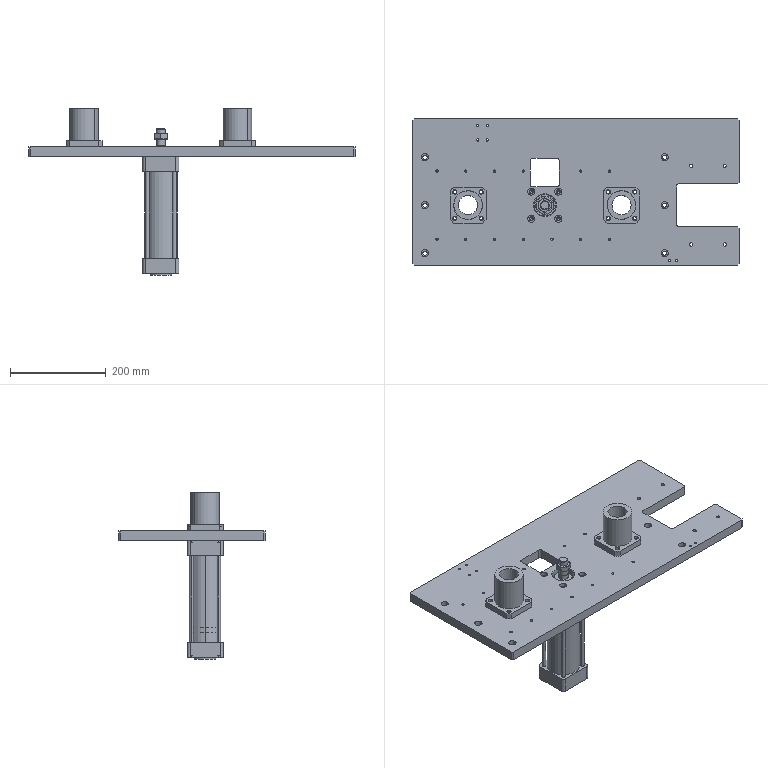Part | SolidWorks | 6 solids | 540 faces | box 680 x 305 x 348 mm | volume 4612161 mm3 | cylinder 256 | plane 180 | cone 78 | torus 24 | spline 2 | commonest cylinder face diameters 5 x38 9 x36 14 x32 6.8 x24 15 x20 6.647 x16